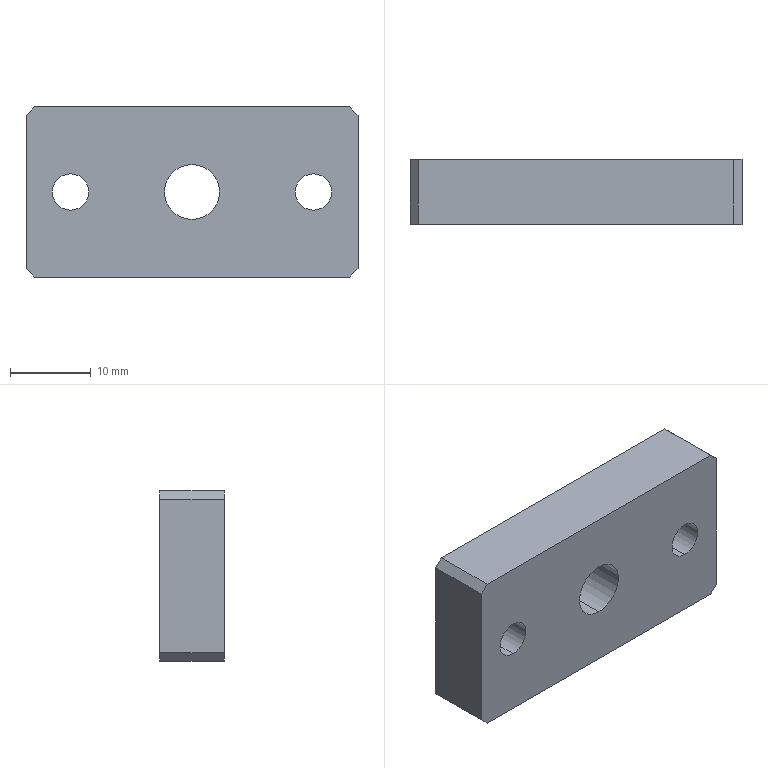Part | NX | features BREP 1 | 1 solid | 22 faces | box 41 x 8 x 21 mm | volume 6018 mm3 | plane 12 | cylinder 10 | commonest cylinder face diameters 4.5 x4 8 x4 6.8 x2
STEP:
#1=CARTESIAN_POINT('',(15.,-4.,-2.25));
#2=VERTEX_POINT('',#1);
#3=CARTESIAN_POINT('',(15.,-4.,2.25));
#4=VERTEX_POINT('',#3);
#5=CARTESIAN_POINT('',(15.,-4.,0.));
#6=DIRECTION('',(0.,1.,0.));
#7=DIRECTION('',(0.,0.,1.));
#8=AXIS2_PLACEMENT_3D('',#5,#6,#7);
#9=CIRCLE('',#8,2.25);
#10=EDGE_CURVE('',#2,#4,#9,.T.);
#11=ORIENTED_EDGE('',*,*,#10,.F.);
#12=CARTESIAN_POINT('',(15.,-0.5,-2.25));
#13=VERTEX_POINT('',#12);
#14=CARTESIAN_POINT('',(15.,4.,-2.25));
#15=DIRECTION('',(0.,1.,0.));
#16=VECTOR('',#15,1000.);
#17=LINE('',#14,#16);
#18=EDGE_CURVE('',#13,#2,#17,.F.);
#19=ORIENTED_EDGE('',*,*,#18,.F.);
#20=CARTESIAN_POINT('',(15.,-0.5,2.25));
#21=VERTEX_POINT('',#20);
#22=CARTESIAN_POINT('',(15.,-0.5,0.));
#23=DIRECTION('',(0.,1.,0.));
#24=DIRECTION('',(0.,0.,1.));
#25=AXIS2_PLACEMENT_3D('',#22,#23,#24);
#26=CIRCLE('',#25,2.25);
#27=EDGE_CURVE('',#13,#21,#26,.T.);
#28=ORIENTED_EDGE('',*,*,#27,.T.);
#29=CARTESIAN_POINT('',(15.,4.,2.25));
#30=DIRECTION('',(0.,1.,0.));
#31=VECTOR('',#30,1000.);
#32=LINE('',#29,#31);
#33=EDGE_CURVE('',#21,#4,#32,.F.);
#34=ORIENTED_EDGE('',*,*,#33,.T.);
#35=EDGE_LOOP('',(#11,#19,#28,#34));
#36=FACE_BOUND('',#35,.T.);
#37=CARTESIAN_POINT('',(15.,4.,0.));
#38=DIRECTION('',(0.,1.,0.));
#39=DIRECTION('',(0.,0.,1.));
#40=AXIS2_PLACEMENT_3D('',#37,#38,#39);
#41=CYLINDRICAL_SURFACE('',#40,2.25);
#42=ADVANCED_FACE('',(#36),#41,.F.);
#43=CARTESIAN_POINT('',(15.,-0.5,-4.));
#44=VERTEX_POINT('',#43);
#45=CARTESIAN_POINT('',(15.,-0.5,4.));
#46=VERTEX_POINT('',#45);
#47=CARTESIAN_POINT('',(15.,-0.5,0.));
#48=DIRECTION('',(0.,1.,0.));
#49=DIRECTION('',(0.,0.,1.));
#50=AXIS2_PLACEMENT_3D('',#47,#48,#49);
#51=CIRCLE('',#50,4.);
#52=EDGE_CURVE('',#44,#46,#51,.T.);
#53=ORIENTED_EDGE('',*,*,#52,.F.);
#54=CARTESIAN_POINT('',(15.,4.,-4.));
#55=VERTEX_POINT('',#54);
#56=CARTESIAN_POINT('',(15.,4.,-4.));
#57=DIRECTION('',(0.,1.,0.));
#58=VECTOR('',#57,1000.);
#59=LINE('',#56,#58);
#60=EDGE_CURVE('',#55,#44,#59,.F.);
#61=ORIENTED_EDGE('',*,*,#60,.F.);
#62=CARTESIAN_POINT('',(15.,4.,4.));
#63=VERTEX_POINT('',#62);
#64=CARTESIAN_POINT('',(15.,4.,0.));
#65=DIRECTION('',(0.,1.,0.));
#66=DIRECTION('',(0.,0.,1.));
#67=AXIS2_PLACEMENT_3D('',#64,#65,#66);
#68=CIRCLE('',#67,4.);
#69=EDGE_CURVE('',#55,#63,#68,.T.);
#70=ORIENTED_EDGE('',*,*,#69,.T.);
#71=CARTESIAN_POINT('',(15.,4.,4.));
#72=DIRECTION('',(0.,1.,0.));
#73=VECTOR('',#72,1000.);
#74=LINE('',#71,#73);
#75=EDGE_CURVE('',#63,#46,#74,.F.);
#76=ORIENTED_EDGE('',*,*,#75,.T.);
#77=EDGE_LOOP('',(#53,#61,#70,#76));
#78=FACE_BOUND('',#77,.T.);
#79=CARTESIAN_POINT('',(15.,4.,0.));
#80=DIRECTION('',(0.,1.,0.));
#81=DIRECTION('',(0.,0.,1.));
#82=AXIS2_PLACEMENT_3D('',#79,#80,#81);
#83=CYLINDRICAL_SURFACE('',#82,4.);
#84=ADVANCED_FACE('',(#78),#83,.F.);
#85=CARTESIAN_POINT('',(-15.,-4.,-2.25));
#86=VERTEX_POINT('',#85);
#87=CARTESIAN_POINT('',(-15.,-4.,2.25));
#88=VERTEX_POINT('',#87);
#89=CARTESIAN_POINT('',(-15.,-4.,0.));
#90=DIRECTION('',(0.,1.,0.));
#91=DIRECTION('',(0.,0.,1.));
#92=AXIS2_PLACEMENT_3D('',#89,#90,#91);
#93=CIRCLE('',#92,2.25);
#94=EDGE_CURVE('',#86,#88,#93,.T.);
#95=ORIENTED_EDGE('',*,*,#94,.F.);
#96=CARTESIAN_POINT('',(-15.,-0.5,-2.25));
#97=VERTEX_POINT('',#96);
#98=CARTESIAN_POINT('',(-15.,4.,-2.25));
#99=DIRECTION('',(0.,1.,0.));
#100=VECTOR('',#99,1000.);
#101=LINE('',#98,#100);
#102=EDGE_CURVE('',#97,#86,#101,.F.);
#103=ORIENTED_EDGE('',*,*,#102,.F.);
#104=CARTESIAN_POINT('',(-15.,-0.5,2.25));
#105=VERTEX_POINT('',#104);
#106=CARTESIAN_POINT('',(-15.,-0.5,0.));
#107=DIRECTION('',(0.,1.,0.));
#108=DIRECTION('',(0.,0.,1.));
#109=AXIS2_PLACEMENT_3D('',#106,#107,#108);
#110=CIRCLE('',#109,2.25);
#111=EDGE_CURVE('',#97,#105,#110,.T.);
#112=ORIENTED_EDGE('',*,*,#111,.T.);
#113=CARTESIAN_POINT('',(-15.,4.,2.25));
#114=DIRECTION('',(0.,1.,0.));
#115=VECTOR('',#114,1000.);
#116=LINE('',#113,#115);
#117=EDGE_CURVE('',#105,#88,#116,.F.);
#118=ORIENTED_EDGE('',*,*,#117,.T.);
#119=EDGE_LOOP('',(#95,#103,#112,#118));
#120=FACE_BOUND('',#119,.T.);
#121=CARTESIAN_POINT('',(-15.,4.,0.));
#122=DIRECTION('',(0.,1.,0.));
#123=DIRECTION('',(0.,0.,1.));
#124=AXIS2_PLACEMENT_3D('',#121,#122,#123);
#125=CYLINDRICAL_SURFACE('',#124,2.25);
#126=ADVANCED_FACE('',(#120),#125,.F.);
#127=CARTESIAN_POINT('',(-15.,-0.5,-4.));
#128=VERTEX_POINT('',#127);
#129=CARTESIAN_POINT('',(-15.,-0.5,4.));
#130=VERTEX_POINT('',#129);
#131=CARTESIAN_POINT('',(-15.,-0.5,0.));
#132=DIRECTION('',(0.,1.,0.));
#133=DIRECTION('',(0.,0.,1.));
#134=AXIS2_PLACEMENT_3D('',#131,#132,#133);
#135=CIRCLE('',#134,4.);
#136=EDGE_CURVE('',#128,#130,#135,.T.);
#137=ORIENTED_EDGE('',*,*,#136,.F.);
#138=CARTESIAN_POINT('',(-15.,4.,-4.));
#139=VERTEX_POINT('',#138);
#140=CARTESIAN_POINT('',(-15.,4.,-4.));
#141=DIRECTION('',(0.,1.,0.));
#142=VECTOR('',#141,1000.);
#143=LINE('',#140,#142);
#144=EDGE_CURVE('',#139,#128,#143,.F.);
#145=ORIENTED_EDGE('',*,*,#144,.F.);
#146=CARTESIAN_POINT('',(-15.,4.,4.));
#147=VERTEX_POINT('',#146);
#148=CARTESIAN_POINT('',(-15.,4.,0.));
#149=DIRECTION('',(0.,1.,0.));
#150=DIRECTION('',(0.,0.,1.));
#151=AXIS2_PLACEMENT_3D('',#148,#149,#150);
#152=CIRCLE('',#151,4.);
#153=EDGE_CURVE('',#139,#147,#152,.T.);
#154=ORIENTED_EDGE('',*,*,#153,.T.);
#155=CARTESIAN_POINT('',(-15.,4.,4.));
#156=DIRECTION('',(0.,1.,0.));
#157=VECTOR('',#156,1000.);
#158=LINE('',#155,#157);
#159=EDGE_CURVE('',#147,#130,#158,.F.);
#160=ORIENTED_EDGE('',*,*,#159,.T.);
#161=EDGE_LOOP('',(#137,#145,#154,#160));
#162=FACE_BOUND('',#161,.T.);
#163=CARTESIAN_POINT('',(-15.,4.,0.));
#164=DIRECTION('',(0.,1.,0.));
#165=DIRECTION('',(0.,0.,1.));
#166=AXIS2_PLACEMENT_3D('',#163,#164,#165);
#167=CYLINDRICAL_SURFACE('',#166,4.);
#168=ADVANCED_FACE('',(#162),#167,.F.);
#169=CARTESIAN_POINT('',(0.,-4.,-3.4));
#170=VERTEX_POINT('',#169);
#171=CARTESIAN_POINT('',(0.,-4.,3.4));
#172=VERTEX_POINT('',#171);
#173=CARTESIAN_POINT('',(0.,-4.,0.));
#174=DIRECTION('',(0.,1.,0.));
#175=DIRECTION('',(0.,0.,1.));
#176=AXIS2_PLACEMENT_3D('',#173,#174,#175);
#177=CIRCLE('',#176,3.4);
#178=EDGE_CURVE('',#170,#172,#177,.T.);
#179=ORIENTED_EDGE('',*,*,#178,.F.);
#180=CARTESIAN_POINT('',(0.,4.,-3.4));
#181=VERTEX_POINT('',#180);
#182=CARTESIAN_POINT('',(0.,4.,-3.4));
#183=DIRECTION('',(0.,1.,0.));
#184=VECTOR('',#183,1000.);
#185=LINE('',#182,#184);
#186=EDGE_CURVE('',#181,#170,#185,.F.);
#187=ORIENTED_EDGE('',*,*,#186,.F.);
#188=CARTESIAN_POINT('',(0.,4.,3.4));
#189=VERTEX_POINT('',#188);
#190=CARTESIAN_POINT('',(0.,4.,0.));
#191=DIRECTION('',(0.,1.,0.));
#192=DIRECTION('',(0.,0.,1.));
#193=AXIS2_PLACEMENT_3D('',#190,#191,#192);
#194=CIRCLE('',#193,3.4);
#195=EDGE_CURVE('',#181,#189,#194,.T.);
#196=ORIENTED_EDGE('',*,*,#195,.T.);
#197=CARTESIAN_POINT('',(0.,4.,3.4));
#198=DIRECTION('',(0.,1.,0.));
#199=VECTOR('',#198,1000.);
#200=LINE('',#197,#199);
#201=EDGE_CURVE('',#189,#172,#200,.F.);
#202=ORIENTED_EDGE('',*,*,#201,.T.);
#203=EDGE_LOOP('',(#179,#187,#196,#202));
#204=FACE_BOUND('',#203,.T.);
#205=CARTESIAN_POINT('',(0.,4.,0.));
#206=DIRECTION('',(0.,1.,0.));
#207=DIRECTION('',(0.,0.,1.));
#208=AXIS2_PLACEMENT_3D('',#205,#206,#207);
#209=CYLINDRICAL_SURFACE('',#208,3.4);
#210=ADVANCED_FACE('',(#204),#209,.F.);
#211=CARTESIAN_POINT('',(19.5,-4.,-10.5));
#212=VERTEX_POINT('',#211);
#213=CARTESIAN_POINT('',(-19.5,-4.,-10.5));
#214=VERTEX_POINT('',#213);
#215=CARTESIAN_POINT('',(20.5,-4.,-10.5));
#216=DIRECTION('',(-1.,0.,0.));
#217=VECTOR('',#216,1000.);
#218=LINE('',#215,#217);
#219=EDGE_CURVE('',#212,#214,#218,.T.);
#220=ORIENTED_EDGE('',*,*,#219,.F.);
#221=CARTESIAN_POINT('',(20.5,-4.,-9.5));
#222=VERTEX_POINT('',#221);
#223=CARTESIAN_POINT('',(20.,-4.,-10.));
#224=DIRECTION('',(0.7071,0.,0.7071));
#225=VECTOR('',#224,1000.);
#226=LINE('',#223,#225);
#227=EDGE_CURVE('',#212,#222,#226,.T.);
#228=ORIENTED_EDGE('',*,*,#227,.T.);
#229=CARTESIAN_POINT('',(20.5,-4.,9.5));
#230=VERTEX_POINT('',#229);
#231=CARTESIAN_POINT('',(20.5,-4.,-10.5));
#232=DIRECTION('',(0.,0.,-1.));
#233=VECTOR('',#232,1000.);
#234=LINE('',#231,#233);
#235=EDGE_CURVE('',#230,#222,#234,.T.);
#236=ORIENTED_EDGE('',*,*,#235,.F.);
#237=CARTESIAN_POINT('',(19.5,-4.,10.5));
#238=VERTEX_POINT('',#237);
#239=CARTESIAN_POINT('',(30.5,-4.,-0.5));
#240=DIRECTION('',(-0.7071,0.,0.7071));
#241=VECTOR('',#240,1000.);
#242=LINE('',#239,#241);
#243=EDGE_CURVE('',#230,#238,#242,.T.);
#244=ORIENTED_EDGE('',*,*,#243,.T.);
#245=CARTESIAN_POINT('',(-19.5,-4.,10.5));
#246=VERTEX_POINT('',#245);
#247=CARTESIAN_POINT('',(20.5,-4.,10.5));
#248=DIRECTION('',(1.,0.,0.));
#249=VECTOR('',#248,1000.);
#250=LINE('',#247,#249);
#251=EDGE_CURVE('',#246,#238,#250,.T.);
#252=ORIENTED_EDGE('',*,*,#251,.F.);
#253=CARTESIAN_POINT('',(-20.5,-4.,9.5));
#254=VERTEX_POINT('',#253);
#255=CARTESIAN_POINT('',(-10.,-4.,20.));
#256=DIRECTION('',(-0.7071,0.,-0.7071));
#257=VECTOR('',#256,1000.);
#258=LINE('',#255,#257);
#259=EDGE_CURVE('',#246,#254,#258,.T.);
#260=ORIENTED_EDGE('',*,*,#259,.T.);
#261=CARTESIAN_POINT('',(-20.5,-4.,-9.5));
#262=VERTEX_POINT('',#261);
#263=CARTESIAN_POINT('',(-20.5,-4.,-10.5));
#264=DIRECTION('',(0.,0.,1.));
#265=VECTOR('',#264,1000.);
#266=LINE('',#263,#265);
#267=EDGE_CURVE('',#262,#254,#266,.T.);
#268=ORIENTED_EDGE('',*,*,#267,.F.);
#269=CARTESIAN_POINT('',(0.5,-4.,-30.5));
#270=DIRECTION('',(0.7071,0.,-0.7071));
#271=VECTOR('',#270,1000.);
#272=LINE('',#269,#271);
#273=EDGE_CURVE('',#262,#214,#272,.T.);
#274=ORIENTED_EDGE('',*,*,#273,.T.);
#275=EDGE_LOOP('',(#220,#228,#236,#244,#252,#260,#268,#274));
#276=FACE_BOUND('',#275,.T.);
#277=CARTESIAN_POINT('',(15.,-4.,0.));
#278=DIRECTION('',(0.,1.,0.));
#279=DIRECTION('',(0.,0.,1.));
#280=AXIS2_PLACEMENT_3D('',#277,#278,#279);
#281=CIRCLE('',#280,2.25);
#282=EDGE_CURVE('',#4,#2,#281,.T.);
#283=ORIENTED_EDGE('',*,*,#282,.T.);
#284=ORIENTED_EDGE('',*,*,#10,.T.);
#285=EDGE_LOOP('',(#283,#284));
#286=FACE_BOUND('',#285,.T.);
#287=CARTESIAN_POINT('',(0.,-4.,0.));
#288=DIRECTION('',(0.,1.,0.));
#289=DIRECTION('',(0.,0.,1.));
#290=AXIS2_PLACEMENT_3D('',#287,#288,#289);
#291=CIRCLE('',#290,3.4);
#292=EDGE_CURVE('',#172,#170,#291,.T.);
#293=ORIENTED_EDGE('',*,*,#292,.T.);
#294=ORIENTED_EDGE('',*,*,#178,.T.);
#295=EDGE_LOOP('',(#293,#294));
#296=FACE_BOUND('',#295,.T.);
#297=CARTESIAN_POINT('',(-15.,-4.,0.));
#298=DIRECTION('',(0.,1.,0.));
#299=DIRECTION('',(0.,0.,1.));
#300=AXIS2_PLACEMENT_3D('',#297,#298,#299);
#301=CIRCLE('',#300,2.25);
#302=EDGE_CURVE('',#88,#86,#301,.T.);
#303=ORIENTED_EDGE('',*,*,#302,.T.);
#304=ORIENTED_EDGE('',*,*,#94,.T.);
#305=EDGE_LOOP('',(#303,#304));
#306=FACE_BOUND('',#305,.T.);
#307=CARTESIAN_POINT('',(20.5,-4.,-10.5));
#308=DIRECTION('',(0.,-1.,0.));
#309=DIRECTION('',(0.,0.,-1.));
#310=AXIS2_PLACEMENT_3D('',#307,#308,#309);
#311=PLANE('',#310);
#312=ADVANCED_FACE('',(#276,#286,#296,#306),#311,.T.);
#313=ORIENTED_EDGE('',*,*,#235,.T.);
#314=CARTESIAN_POINT('',(20.5,4.,-9.5));
#315=VERTEX_POINT('',#314);
#316=CARTESIAN_POINT('',(20.5,4.,-9.5));
#317=DIRECTION('',(0.,1.,0.));
#318=VECTOR('',#317,1000.);
#319=LINE('',#316,#318);
#320=EDGE_CURVE('',#222,#315,#319,.T.);
#321=ORIENTED_EDGE('',*,*,#320,.T.);
#322=CARTESIAN_POINT('',(20.5,4.,9.5));
#323=VERTEX_POINT('',#322);
#324=CARTESIAN_POINT('',(20.5,4.,-10.5));
#325=DIRECTION('',(0.,0.,-1.));
#326=VECTOR('',#325,1000.);
#327=LINE('',#324,#326);
#328=EDGE_CURVE('',#323,#315,#327,.T.);
#329=ORIENTED_EDGE('',*,*,#328,.F.);
#330=CARTESIAN_POINT('',(20.5,4.,9.5));
#331=DIRECTION('',(0.,-1.,0.));
#332=VECTOR('',#331,1000.);
#333=LINE('',#330,#332);
#334=EDGE_CURVE('',#323,#230,#333,.T.);
#335=ORIENTED_EDGE('',*,*,#334,.T.);
#336=EDGE_LOOP('',(#313,#321,#329,#335));
#337=FACE_BOUND('',#336,.T.);
#338=CARTESIAN_POINT('',(20.5,4.,-10.5));
#339=DIRECTION('',(-1.,0.,0.));
#340=DIRECTION('',(0.,0.,1.));
#341=AXIS2_PLACEMENT_3D('',#338,#339,#340);
#342=PLANE('',#341);
#343=ADVANCED_FACE('',(#337),#342,.F.);
#344=CARTESIAN_POINT('',(19.5,4.,-10.5));
#345=VERTEX_POINT('',#344);
#346=CARTESIAN_POINT('',(-19.5,4.,-10.5));
#347=VERTEX_POINT('',#346);
#348=CARTESIAN_POINT('',(20.5,4.,-10.5));
#349=DIRECTION('',(-1.,0.,0.));
#350=VECTOR('',#349,1000.);
#351=LINE('',#348,#350);
#352=EDGE_CURVE('',#345,#347,#351,.T.);
#353=ORIENTED_EDGE('',*,*,#352,.F.);
#354=CARTESIAN_POINT('',(19.5,4.,-10.5));
#355=DIRECTION('',(0.,-1.,0.));
#356=VECTOR('',#355,1000.);
#357=LINE('',#354,#356);
#358=EDGE_CURVE('',#345,#212,#357,.T.);
#359=ORIENTED_EDGE('',*,*,#358,.T.);
#360=ORIENTED_EDGE('',*,*,#219,.T.);
#361=CARTESIAN_POINT('',(-19.5,4.,-10.5));
#362=DIRECTION('',(0.,1.,0.));
#363=VECTOR('',#362,1000.);
#364=LINE('',#361,#363);
#365=EDGE_CURVE('',#214,#347,#364,.T.);
#366=ORIENTED_EDGE('',*,*,#365,.T.);
#367=EDGE_LOOP('',(#353,#359,#360,#366));
#368=FACE_BOUND('',#367,.T.);
#369=CARTESIAN_POINT('',(20.5,4.,-10.5));
#370=DIRECTION('',(0.,0.,1.));
#371=DIRECTION('',(1.,0.,0.));
#372=AXIS2_PLACEMENT_3D('',#369,#370,#371);
#373=PLANE('',#372);
#374=ADVANCED_FACE('',(#368),#373,.F.);
#375=CARTESIAN_POINT('',(-20.5,4.,-9.5));
#376=VERTEX_POINT('',#375);
#377=CARTESIAN_POINT('',(-20.5,4.,9.5));
#378=VERTEX_POINT('',#377);
#379=CARTESIAN_POINT('',(-20.5,4.,-10.5));
#380=DIRECTION('',(0.,0.,1.));
#381=VECTOR('',#380,1000.);
#382=LINE('',#379,#381);
#383=EDGE_CURVE('',#376,#378,#382,.T.);
#384=ORIENTED_EDGE('',*,*,#383,.F.);
#385=CARTESIAN_POINT('',(-20.5,4.,-9.5));
#386=DIRECTION('',(0.,-1.,0.));
#387=VECTOR('',#386,1000.);
#388=LINE('',#385,#387);
#389=EDGE_CURVE('',#376,#262,#388,.T.);
#390=ORIENTED_EDGE('',*,*,#389,.T.);
#391=ORIENTED_EDGE('',*,*,#267,.T.);
#392=CARTESIAN_POINT('',(-20.5,4.,9.5));
#393=DIRECTION('',(0.,1.,0.));
#394=VECTOR('',#393,1000.);
#395=LINE('',#392,#394);
#396=EDGE_CURVE('',#254,#378,#395,.T.);
#397=ORIENTED_EDGE('',*,*,#396,.T.);
#398=EDGE_LOOP('',(#384,#390,#391,#397));
#399=FACE_BOUND('',#398,.T.);
#400=CARTESIAN_POINT('',(-20.5,4.,-10.5));
#401=DIRECTION('',(1.,0.,0.));
#402=DIRECTION('',(0.,1.,0.));
#403=AXIS2_PLACEMENT_3D('',#400,#401,#402);
#404=PLANE('',#403);
#405=ADVANCED_FACE('',(#399),#404,.F.);
#406=ORIENTED_EDGE('',*,*,#251,.T.);
#407=CARTESIAN_POINT('',(19.5,4.,10.5));
#408=VERTEX_POINT('',#407);
#409=CARTESIAN_POINT('',(19.5,4.,10.5));
#410=DIRECTION('',(0.,1.,0.));
#411=VECTOR('',#410,1000.);
#412=LINE('',#409,#411);
#413=EDGE_CURVE('',#238,#408,#412,.T.);
#414=ORIENTED_EDGE('',*,*,#413,.T.);
#415=CARTESIAN_POINT('',(-19.5,4.,10.5));
#416=VERTEX_POINT('',#415);
#417=CARTESIAN_POINT('',(20.5,4.,10.5));
#418=DIRECTION('',(1.,0.,0.));
#419=VECTOR('',#418,1000.);
#420=LINE('',#417,#419);
#421=EDGE_CURVE('',#416,#408,#420,.T.);
#422=ORIENTED_EDGE('',*,*,#421,.F.);
#423=CARTESIAN_POINT('',(-19.5,4.,10.5));
#424=DIRECTION('',(0.,-1.,0.));
#425=VECTOR('',#424,1000.);
#426=LINE('',#423,#425);
#427=EDGE_CURVE('',#416,#246,#426,.T.);
#428=ORIENTED_EDGE('',*,*,#427,.T.);
#429=EDGE_LOOP('',(#406,#414,#422,#428));
#430=FACE_BOUND('',#429,.T.);
#431=CARTESIAN_POINT('',(20.5,4.,10.5));
#432=DIRECTION('',(0.,0.,-1.));
#433=DIRECTION('',(-1.,0.,0.));
#434=AXIS2_PLACEMENT_3D('',#431,#432,#433);
#435=PLANE('',#434);
#436=ADVANCED_FACE('',(#430),#435,.F.);
#437=ORIENTED_EDGE('',*,*,#328,.T.);
#438=CARTESIAN_POINT('',(19.5,4.,-10.5));
#439=DIRECTION('',(-0.7071,0.,-0.7071));
#440=VECTOR('',#439,1000.);
#441=LINE('',#438,#440);
#442=EDGE_CURVE('',#315,#345,#441,.T.);
#443=ORIENTED_EDGE('',*,*,#442,.T.);
#444=ORIENTED_EDGE('',*,*,#352,.T.);
#445=CARTESIAN_POINT('',(-20.5,4.,-9.5));
#446=DIRECTION('',(-0.7071,0.,0.7071));
#447=VECTOR('',#446,1000.);
#448=LINE('',#445,#447);
#449=EDGE_CURVE('',#347,#376,#448,.T.);
#450=ORIENTED_EDGE('',*,*,#449,.T.);
#451=ORIENTED_EDGE('',*,*,#383,.T.);
#452=CARTESIAN_POINT('',(-19.5,4.,10.5));
#453=DIRECTION('',(0.7071,0.,0.7071));
#454=VECTOR('',#453,1000.);
#455=LINE('',#452,#454);
#456=EDGE_CURVE('',#378,#416,#455,.T.);
#457=ORIENTED_EDGE('',*,*,#456,.T.);
#458=ORIENTED_EDGE('',*,*,#421,.T.);
#459=CARTESIAN_POINT('',(20.5,4.,9.5));
#460=DIRECTION('',(0.7071,0.,-0.7071));
#461=VECTOR('',#460,1000.);
#462=LINE('',#459,#461);
#463=EDGE_CURVE('',#408,#323,#462,.T.);
#464=ORIENTED_EDGE('',*,*,#463,.T.);
#465=EDGE_LOOP('',(#437,#443,#444,#450,#451,#457,#458,#464));
#466=FACE_BOUND('',#465,.T.);
#467=CARTESIAN_POINT('',(15.,4.,0.));
#468=DIRECTION('',(0.,1.,0.));
#469=DIRECTION('',(0.,0.,1.));
#470=AXIS2_PLACEMENT_3D('',#467,#468,#469);
#471=CIRCLE('',#470,4.);
#472=EDGE_CURVE('',#63,#55,#471,.T.);
#473=ORIENTED_EDGE('',*,*,#472,.F.);
#474=ORIENTED_EDGE('',*,*,#69,.F.);
#475=EDGE_LOOP('',(#473,#474));
#476=FACE_BOUND('',#475,.T.);
#477=CARTESIAN_POINT('',(-15.,4.,0.));
#478=DIRECTION('',(0.,1.,0.));
#479=DIRECTION('',(0.,0.,1.));
#480=AXIS2_PLACEMENT_3D('',#477,#478,#479);
#481=CIRCLE('',#480,4.);
#482=EDGE_CURVE('',#147,#139,#481,.T.);
#483=ORIENTED_EDGE('',*,*,#482,.F.);
#484=ORIENTED_EDGE('',*,*,#153,.F.);
#485=EDGE_LOOP('',(#483,#484));
#486=FACE_BOUND('',#485,.T.);
#487=CARTESIAN_POINT('',(0.,4.,0.));
#488=DIRECTION('',(0.,1.,0.));
#489=DIRECTION('',(0.,0.,1.));
#490=AXIS2_PLACEMENT_3D('',#487,#488,#489);
#491=CIRCLE('',#490,3.4);
#492=EDGE_CURVE('',#189,#181,#491,.T.);
#493=ORIENTED_EDGE('',*,*,#492,.F.);
#494=ORIENTED_EDGE('',*,*,#195,.F.);
#495=EDGE_LOOP('',(#493,#494));
#496=FACE_BOUND('',#495,.T.);
#497=CARTESIAN_POINT('',(20.5,4.,-10.5));
#498=DIRECTION('',(0.,-1.,0.));
#499=DIRECTION('',(0.,0.,-1.));
#500=AXIS2_PLACEMENT_3D('',#497,#498,#499);
#501=PLANE('',#500);
#502=ADVANCED_FACE('',(#466,#476,#486,#496),#501,.F.);
#503=ORIENTED_EDGE('',*,*,#442,.F.);
#504=ORIENTED_EDGE('',*,*,#320,.F.);
#505=ORIENTED_EDGE('',*,*,#227,.F.);
#506=ORIENTED_EDGE('',*,*,#358,.F.);
#507=EDGE_LOOP('',(#503,#504,#505,#506));
#508=FACE_BOUND('',#507,.T.);
#509=CARTESIAN_POINT('',(19.5,4.,-10.5));
#510=DIRECTION('',(-0.7071,0.,0.7071));
#511=DIRECTION('',(0.,1.,0.));
#512=AXIS2_PLACEMENT_3D('',#509,#510,#511);
#513=PLANE('',#512);
#514=ADVANCED_FACE('',(#508),#513,.F.);
#515=ORIENTED_EDGE('',*,*,#463,.F.);
#516=ORIENTED_EDGE('',*,*,#413,.F.);
#517=ORIENTED_EDGE('',*,*,#243,.F.);
#518=ORIENTED_EDGE('',*,*,#334,.F.);
#519=EDGE_LOOP('',(#515,#516,#517,#518));
#520=FACE_BOUND('',#519,.T.);
#521=CARTESIAN_POINT('',(20.5,4.,9.5));
#522=DIRECTION('',(-0.7071,0.,-0.7071));
#523=DIRECTION('',(-0.7071,0.,0.7071));
#524=AXIS2_PLACEMENT_3D('',#521,#522,#523);
#525=PLANE('',#524);
#526=ADVANCED_FACE('',(#520),#525,.F.);
#527=ORIENTED_EDGE('',*,*,#449,.F.);
#528=ORIENTED_EDGE('',*,*,#365,.F.);
#529=ORIENTED_EDGE('',*,*,#273,.F.);
#530=ORIENTED_EDGE('',*,*,#389,.F.);
#531=EDGE_LOOP('',(#527,#528,#529,#530));
#532=FACE_BOUND('',#531,.T.);
#533=CARTESIAN_POINT('',(-20.5,4.,-9.5));
#534=DIRECTION('',(0.7071,0.,0.7071));
#535=DIRECTION('',(0.,-1.,0.));
#536=AXIS2_PLACEMENT_3D('',#533,#534,#535);
#537=PLANE('',#536);
#538=ADVANCED_FACE('',(#532),#537,.F.);
#539=ORIENTED_EDGE('',*,*,#456,.F.);
#540=ORIENTED_EDGE('',*,*,#396,.F.);
#541=ORIENTED_EDGE('',*,*,#259,.F.);
#542=ORIENTED_EDGE('',*,*,#427,.F.);
#543=EDGE_LOOP('',(#539,#540,#541,#542));
#544=FACE_BOUND('',#543,.T.);
#545=CARTESIAN_POINT('',(-19.5,4.,10.5));
#546=DIRECTION('',(0.7071,0.,-0.7071));
#547=DIRECTION('',(0.,-1.,0.));
#548=AXIS2_PLACEMENT_3D('',#545,#546,#547);
#549=PLANE('',#548);
#550=ADVANCED_FACE('',(#544),#549,.F.);
#551=ORIENTED_EDGE('',*,*,#186,.T.);
#552=ORIENTED_EDGE('',*,*,#292,.F.);
#553=ORIENTED_EDGE('',*,*,#201,.F.);
#554=ORIENTED_EDGE('',*,*,#492,.T.);
#555=EDGE_LOOP('',(#551,#552,#553,#554));
#556=FACE_BOUND('',#555,.T.);
#557=CARTESIAN_POINT('',(0.,4.,0.));
#558=DIRECTION('',(0.,1.,0.));
#559=DIRECTION('',(0.,0.,1.));
#560=AXIS2_PLACEMENT_3D('',#557,#558,#559);
#561=CYLINDRICAL_SURFACE('',#560,3.4);
#562=ADVANCED_FACE('',(#556),#561,.F.);
#563=ORIENTED_EDGE('',*,*,#144,.T.);
#564=CARTESIAN_POINT('',(-15.,-0.5,0.));
#565=DIRECTION('',(0.,1.,0.));
#566=DIRECTION('',(0.,0.,1.));
#567=AXIS2_PLACEMENT_3D('',#564,#565,#566);
#568=CIRCLE('',#567,4.);
#569=EDGE_CURVE('',#130,#128,#568,.T.);
#570=ORIENTED_EDGE('',*,*,#569,.F.);
#571=ORIENTED_EDGE('',*,*,#159,.F.);
#572=ORIENTED_EDGE('',*,*,#482,.T.);
#573=EDGE_LOOP('',(#563,#570,#571,#572));
#574=FACE_BOUND('',#573,.T.);
#575=CARTESIAN_POINT('',(-15.,4.,0.));
#576=DIRECTION('',(0.,1.,0.));
#577=DIRECTION('',(0.,0.,1.));
#578=AXIS2_PLACEMENT_3D('',#575,#576,#577);
#579=CYLINDRICAL_SURFACE('',#578,4.);
#580=ADVANCED_FACE('',(#574),#579,.F.);
#581=ORIENTED_EDGE('',*,*,#569,.T.);
#582=ORIENTED_EDGE('',*,*,#136,.T.);
#583=EDGE_LOOP('',(#581,#582));
#584=FACE_BOUND('',#583,.T.);
#585=CARTESIAN_POINT('',(-15.,-0.5,0.));
#586=DIRECTION('',(0.,1.,0.));
#587=DIRECTION('',(0.,0.,1.));
#588=AXIS2_PLACEMENT_3D('',#585,#586,#587);
#589=CIRCLE('',#588,2.25);
#590=EDGE_CURVE('',#105,#97,#589,.T.);
#591=ORIENTED_EDGE('',*,*,#590,.F.);
#592=ORIENTED_EDGE('',*,*,#111,.F.);
#593=EDGE_LOOP('',(#591,#592));
#594=FACE_BOUND('',#593,.T.);
#595=CARTESIAN_POINT('',(-12.75,-0.5,0.));
#596=DIRECTION('',(0.,-1.,0.));
#597=DIRECTION('',(0.,0.,-1.));
#598=AXIS2_PLACEMENT_3D('',#595,#596,#597);
#599=PLANE('',#598);
#600=ADVANCED_FACE('',(#584,#594),#599,.F.);
#601=ORIENTED_EDGE('',*,*,#102,.T.);
#602=ORIENTED_EDGE('',*,*,#302,.F.);
#603=ORIENTED_EDGE('',*,*,#117,.F.);
#604=ORIENTED_EDGE('',*,*,#590,.T.);
#605=EDGE_LOOP('',(#601,#602,#603,#604));
#606=FACE_BOUND('',#605,.T.);
#607=CARTESIAN_POINT('',(-15.,4.,0.));
#608=DIRECTION('',(0.,1.,0.));
#609=DIRECTION('',(0.,0.,1.));
#610=AXIS2_PLACEMENT_3D('',#607,#608,#609);
#611=CYLINDRICAL_SURFACE('',#610,2.25);
#612=ADVANCED_FACE('',(#606),#611,.F.);
#613=ORIENTED_EDGE('',*,*,#60,.T.);
#614=CARTESIAN_POINT('',(15.,-0.5,0.));
#615=DIRECTION('',(0.,1.,0.));
#616=DIRECTION('',(0.,0.,1.));
#617=AXIS2_PLACEMENT_3D('',#614,#615,#616);
#618=CIRCLE('',#617,4.);
#619=EDGE_CURVE('',#46,#44,#618,.T.);
#620=ORIENTED_EDGE('',*,*,#619,.F.);
#621=ORIENTED_EDGE('',*,*,#75,.F.);
#622=ORIENTED_EDGE('',*,*,#472,.T.);
#623=EDGE_LOOP('',(#613,#620,#621,#622));
#624=FACE_BOUND('',#623,.T.);
#625=CARTESIAN_POINT('',(15.,4.,0.));
#626=DIRECTION('',(0.,1.,0.));
#627=DIRECTION('',(0.,0.,1.));
#628=AXIS2_PLACEMENT_3D('',#625,#626,#627);
#629=CYLINDRICAL_SURFACE('',#628,4.);
#630=ADVANCED_FACE('',(#624),#629,.F.);
#631=ORIENTED_EDGE('',*,*,#619,.T.);
#632=ORIENTED_EDGE('',*,*,#52,.T.);
#633=EDGE_LOOP('',(#631,#632));
#634=FACE_BOUND('',#633,.T.);
#635=CARTESIAN_POINT('',(15.,-0.5,0.));
#636=DIRECTION('',(0.,1.,0.));
#637=DIRECTION('',(0.,0.,1.));
#638=AXIS2_PLACEMENT_3D('',#635,#636,#637);
#639=CIRCLE('',#638,2.25);
#640=EDGE_CURVE('',#21,#13,#639,.T.);
#641=ORIENTED_EDGE('',*,*,#640,.F.);
#642=ORIENTED_EDGE('',*,*,#27,.F.);
#643=EDGE_LOOP('',(#641,#642));
#644=FACE_BOUND('',#643,.T.);
#645=CARTESIAN_POINT('',(17.25,-0.5,0.));
#646=DIRECTION('',(0.,-1.,0.));
#647=DIRECTION('',(0.,0.,-1.));
#648=AXIS2_PLACEMENT_3D('',#645,#646,#647);
#649=PLANE('',#648);
#650=ADVANCED_FACE('',(#634,#644),#649,.F.);
#651=ORIENTED_EDGE('',*,*,#18,.T.);
#652=ORIENTED_EDGE('',*,*,#282,.F.);
#653=ORIENTED_EDGE('',*,*,#33,.F.);
#654=ORIENTED_EDGE('',*,*,#640,.T.);
#655=EDGE_LOOP('',(#651,#652,#653,#654));
#656=FACE_BOUND('',#655,.T.);
#657=CARTESIAN_POINT('',(15.,4.,0.));
#658=DIRECTION('',(0.,1.,0.));
#659=DIRECTION('',(0.,0.,1.));
#660=AXIS2_PLACEMENT_3D('',#657,#658,#659);
#661=CYLINDRICAL_SURFACE('',#660,2.25);
#662=ADVANCED_FACE('',(#656),#661,.F.);
#663=CLOSED_SHELL('',(#42,#84,#126,#168,#210,#312,#343,#374,#405,#436,#502,#514,#526,#538,#550,#562,#580,#600,#612,#630,#650,#662));
#664=MANIFOLD_SOLID_BREP('',#663);
#665=(LENGTH_UNIT()NAMED_UNIT(*)SI_UNIT(.MILLI.,.METRE.));
#666=UNCERTAINTY_MEASURE_WITH_UNIT(LENGTH_MEASURE(0.00001),#665,'','');
#667=(NAMED_UNIT(*)PLANE_ANGLE_UNIT()SI_UNIT($,.RADIAN.));
#668=(NAMED_UNIT(*)SI_UNIT($,.STERADIAN.)SOLID_ANGLE_UNIT());
#669=(GEOMETRIC_REPRESENTATION_CONTEXT(3)GLOBAL_UNCERTAINTY_ASSIGNED_CONTEXT((#666))GLOBAL_UNIT_ASSIGNED_CONTEXT((#665,#667,#668))REPRESENTATION_CONTEXT('',''));
#670=ADVANCED_BREP_SHAPE_REPRESENTATION('',(#664),#669);